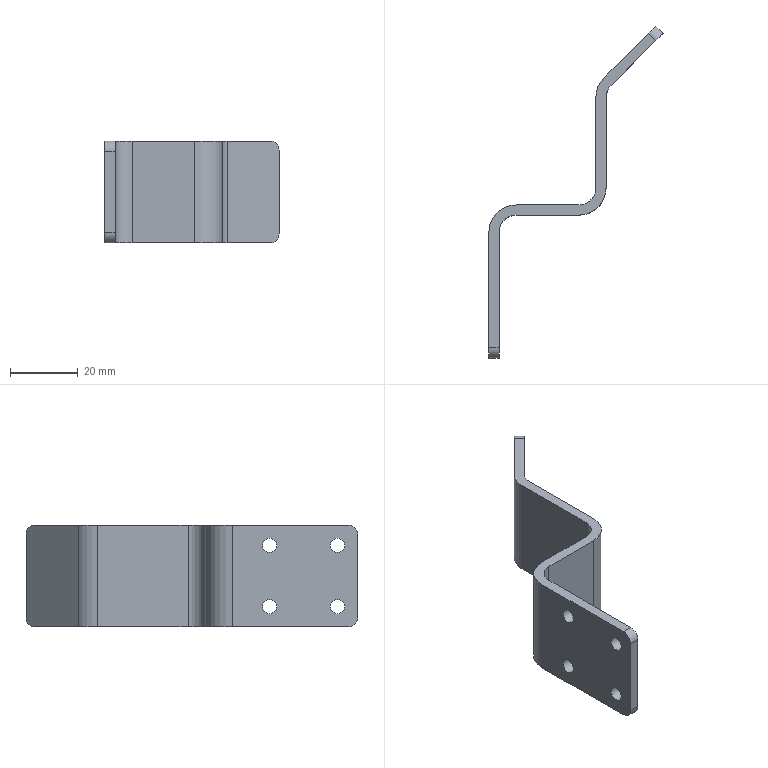Part | NX | features BREP 1 | 1 solid | 26 faces | box 51.299 x 97.678 x 30 mm | volume 11456 mm3 | cylinder 14 | plane 12 | commonest cylinder face diameters 4.2 x4 6 x4 10 x3 16 x3
STEP:
#1=CARTESIAN_POINT('',(-31.5,-50.,3.));
#2=VERTEX_POINT('',#1);
#3=CARTESIAN_POINT('',(-31.5,-47.,0.));
#4=VERTEX_POINT('',#3);
#5=CARTESIAN_POINT('',(-31.5,-47.,3.));
#6=DIRECTION('',(1.,0.,0.));
#7=DIRECTION('',(0.,1.,0.));
#8=AXIS2_PLACEMENT_3D('',#5,#6,#7);
#9=CIRCLE('',#8,3.);
#10=EDGE_CURVE('',#2,#4,#9,.T.);
#11=ORIENTED_EDGE('',*,*,#10,.F.);
#12=CARTESIAN_POINT('',(-31.5,-50.,27.));
#13=VERTEX_POINT('',#12);
#14=CARTESIAN_POINT('',(-31.5,-50.,0.));
#15=DIRECTION('',(0.,0.,-1.));
#16=VECTOR('',#15,1000.);
#17=LINE('',#14,#16);
#18=EDGE_CURVE('',#13,#2,#17,.T.);
#19=ORIENTED_EDGE('',*,*,#18,.F.);
#20=CARTESIAN_POINT('',(-31.5,-47.,30.));
#21=VERTEX_POINT('',#20);
#22=CARTESIAN_POINT('',(-31.5,-47.,27.));
#23=DIRECTION('',(1.,0.,0.));
#24=DIRECTION('',(0.,1.,0.));
#25=AXIS2_PLACEMENT_3D('',#22,#23,#24);
#26=CIRCLE('',#25,3.);
#27=EDGE_CURVE('',#21,#13,#26,.T.);
#28=ORIENTED_EDGE('',*,*,#27,.F.);
#29=CARTESIAN_POINT('',(-31.5,-13.,30.));
#30=VERTEX_POINT('',#29);
#31=CARTESIAN_POINT('',(-31.5,0.,30.));
#32=DIRECTION('',(0.,-1.,0.));
#33=VECTOR('',#32,1000.);
#34=LINE('',#31,#33);
#35=EDGE_CURVE('',#30,#21,#34,.T.);
#36=ORIENTED_EDGE('',*,*,#35,.F.);
#37=CARTESIAN_POINT('',(-31.5,-13.,0.));
#38=VERTEX_POINT('',#37);
#39=CARTESIAN_POINT('',(-31.5,-13.,0.));
#40=DIRECTION('',(0.,0.,1.));
#41=VECTOR('',#40,1000.);
#42=LINE('',#39,#41);
#43=EDGE_CURVE('',#38,#30,#42,.T.);
#44=ORIENTED_EDGE('',*,*,#43,.F.);
#45=CARTESIAN_POINT('',(-31.5,0.,0.));
#46=DIRECTION('',(0.,1.,0.));
#47=VECTOR('',#46,1000.);
#48=LINE('',#45,#47);
#49=EDGE_CURVE('',#4,#38,#48,.T.);
#50=ORIENTED_EDGE('',*,*,#49,.F.);
#51=EDGE_LOOP('',(#11,#19,#28,#36,#44,#50));
#52=FACE_BOUND('',#51,.T.);
#53=CARTESIAN_POINT('',(-31.5,-44.,26.1));
#54=VERTEX_POINT('',#53);
#55=CARTESIAN_POINT('',(-31.5,-44.,24.));
#56=DIRECTION('',(-1.,0.,0.));
#57=DIRECTION('',(0.,0.,1.));
#58=AXIS2_PLACEMENT_3D('',#55,#56,#57);
#59=CIRCLE('',#58,2.1);
#60=EDGE_CURVE('',#54,#54,#59,.T.);
#61=ORIENTED_EDGE('',*,*,#60,.F.);
#62=EDGE_LOOP('',(#61));
#63=FACE_BOUND('',#62,.T.);
#64=CARTESIAN_POINT('',(-31.5,-24.,26.1));
#65=VERTEX_POINT('',#64);
#66=CARTESIAN_POINT('',(-31.5,-24.,24.));
#67=DIRECTION('',(-1.,0.,0.));
#68=DIRECTION('',(0.,0.,1.));
#69=AXIS2_PLACEMENT_3D('',#66,#67,#68);
#70=CIRCLE('',#69,2.1);
#71=EDGE_CURVE('',#65,#65,#70,.T.);
#72=ORIENTED_EDGE('',*,*,#71,.F.);
#73=EDGE_LOOP('',(#72));
#74=FACE_BOUND('',#73,.T.);
#75=CARTESIAN_POINT('',(-31.5,-44.,8.1));
#76=VERTEX_POINT('',#75);
#77=CARTESIAN_POINT('',(-31.5,-44.,6.));
#78=DIRECTION('',(-1.,0.,0.));
#79=DIRECTION('',(0.,0.,1.));
#80=AXIS2_PLACEMENT_3D('',#77,#78,#79);
#81=CIRCLE('',#80,2.1);
#82=EDGE_CURVE('',#76,#76,#81,.T.);
#83=ORIENTED_EDGE('',*,*,#82,.F.);
#84=EDGE_LOOP('',(#83));
#85=FACE_BOUND('',#84,.T.);
#86=CARTESIAN_POINT('',(-31.5,-24.,8.1));
#87=VERTEX_POINT('',#86);
#88=CARTESIAN_POINT('',(-31.5,-24.,6.));
#89=DIRECTION('',(-1.,0.,0.));
#90=DIRECTION('',(0.,0.,1.));
#91=AXIS2_PLACEMENT_3D('',#88,#89,#90);
#92=CIRCLE('',#91,2.1);
#93=EDGE_CURVE('',#87,#87,#92,.T.);
#94=ORIENTED_EDGE('',*,*,#93,.F.);
#95=EDGE_LOOP('',(#94));
#96=FACE_BOUND('',#95,.T.);
#97=CARTESIAN_POINT('',(-31.5,0.,0.));
#98=DIRECTION('',(1.,0.,0.));
#99=DIRECTION('',(0.,0.,1.));
#100=AXIS2_PLACEMENT_3D('',#97,#98,#99);
#101=PLANE('',#100);
#102=ADVANCED_FACE('',(#52,#63,#74,#85,#96),#101,.F.);
#103=CARTESIAN_POINT('',(-28.5,-47.,0.));
#104=VERTEX_POINT('',#103);
#105=CARTESIAN_POINT('',(-31.5,-47.,0.));
#106=DIRECTION('',(1.,0.,0.));
#107=VECTOR('',#106,1000.);
#108=LINE('',#105,#107);
#109=EDGE_CURVE('',#4,#104,#108,.T.);
#110=ORIENTED_EDGE('',*,*,#109,.F.);
#111=ORIENTED_EDGE('',*,*,#49,.T.);
#112=CARTESIAN_POINT('',(-23.5,-5.,0.));
#113=VERTEX_POINT('',#112);
#114=CARTESIAN_POINT('',(-23.5,-13.,0.));
#115=DIRECTION('',(0.,0.,1.));
#116=DIRECTION('',(-1.,0.,0.));
#117=AXIS2_PLACEMENT_3D('',#114,#115,#116);
#118=CIRCLE('',#117,8.);
#119=EDGE_CURVE('',#113,#38,#118,.T.);
#120=ORIENTED_EDGE('',*,*,#119,.F.);
#121=CARTESIAN_POINT('',(-5.,-5.,0.));
#122=VERTEX_POINT('',#121);
#123=CARTESIAN_POINT('',(0.,-5.,0.));
#124=DIRECTION('',(-1.,0.,0.));
#125=VECTOR('',#124,1000.);
#126=LINE('',#123,#125);
#127=EDGE_CURVE('',#122,#113,#126,.T.);
#128=ORIENTED_EDGE('',*,*,#127,.F.);
#129=CARTESIAN_POINT('',(0.,0.,0.));
#130=VERTEX_POINT('',#129);
#131=CARTESIAN_POINT('',(-5.,0.,0.));
#132=DIRECTION('',(0.,0.,1.));
#133=DIRECTION('',(1.,0.,0.));
#134=AXIS2_PLACEMENT_3D('',#131,#132,#133);
#135=CIRCLE('',#134,5.);
#136=EDGE_CURVE('',#122,#130,#135,.T.);
#137=ORIENTED_EDGE('',*,*,#136,.T.);
#138=CARTESIAN_POINT('',(0.,26.686,0.));
#139=VERTEX_POINT('',#138);
#140=CARTESIAN_POINT('',(0.,0.,0.));
#141=DIRECTION('',(0.,-1.,0.));
#142=VECTOR('',#141,1000.);
#143=LINE('',#140,#142);
#144=EDGE_CURVE('',#139,#130,#143,.T.);
#145=ORIENTED_EDGE('',*,*,#144,.F.);
#146=CARTESIAN_POINT('',(2.343,32.343,0.));
#147=VERTEX_POINT('',#146);
#148=CARTESIAN_POINT('',(8.,26.686,0.));
#149=DIRECTION('',(0.,0.,1.));
#150=DIRECTION('',(-1.,0.,0.));
#151=AXIS2_PLACEMENT_3D('',#148,#149,#150);
#152=CIRCLE('',#151,8.);
#153=EDGE_CURVE('',#147,#139,#152,.T.);
#154=ORIENTED_EDGE('',*,*,#153,.F.);
#155=CARTESIAN_POINT('',(15.556,45.556,0.));
#156=VERTEX_POINT('',#155);
#157=CARTESIAN_POINT('',(0.,30.,0.));
#158=DIRECTION('',(-0.7071,-0.7071,0.));
#159=VECTOR('',#158,1000.);
#160=LINE('',#157,#159);
#161=EDGE_CURVE('',#156,#147,#160,.T.);
#162=ORIENTED_EDGE('',*,*,#161,.F.);
#163=CARTESIAN_POINT('',(17.678,43.435,0.));
#164=VERTEX_POINT('',#163);
#165=CARTESIAN_POINT('',(15.556,45.556,0.));
#166=DIRECTION('',(0.7071,-0.7071,0.));
#167=VECTOR('',#166,1000.);
#168=LINE('',#165,#167);
#169=EDGE_CURVE('',#156,#164,#168,.T.);
#170=ORIENTED_EDGE('',*,*,#169,.T.);
#171=CARTESIAN_POINT('',(4.464,30.222,0.));
#172=VERTEX_POINT('',#171);
#173=CARTESIAN_POINT('',(17.678,43.435,0.));
#174=DIRECTION('',(-0.7071,-0.7071,0.));
#175=VECTOR('',#174,1000.);
#176=LINE('',#173,#175);
#177=EDGE_CURVE('',#164,#172,#176,.T.);
#178=ORIENTED_EDGE('',*,*,#177,.T.);
#179=CARTESIAN_POINT('',(3.,26.686,0.));
#180=VERTEX_POINT('',#179);
#181=CARTESIAN_POINT('',(8.,26.686,0.));
#182=DIRECTION('',(0.,0.,1.));
#183=DIRECTION('',(-1.,0.,0.));
#184=AXIS2_PLACEMENT_3D('',#181,#182,#183);
#185=CIRCLE('',#184,5.);
#186=EDGE_CURVE('',#172,#180,#185,.T.);
#187=ORIENTED_EDGE('',*,*,#186,.T.);
#188=CARTESIAN_POINT('',(3.,0.,0.));
#189=VERTEX_POINT('',#188);
#190=CARTESIAN_POINT('',(3.,30.222,0.));
#191=DIRECTION('',(0.,-1.,0.));
#192=VECTOR('',#191,1000.);
#193=LINE('',#190,#192);
#194=EDGE_CURVE('',#180,#189,#193,.T.);
#195=ORIENTED_EDGE('',*,*,#194,.T.);
#196=CARTESIAN_POINT('',(-5.,-8.,0.));
#197=VERTEX_POINT('',#196);
#198=CARTESIAN_POINT('',(-5.,0.,0.));
#199=DIRECTION('',(0.,0.,-1.));
#200=DIRECTION('',(1.,0.,0.));
#201=AXIS2_PLACEMENT_3D('',#198,#199,#200);
#202=CIRCLE('',#201,8.);
#203=EDGE_CURVE('',#189,#197,#202,.T.);
#204=ORIENTED_EDGE('',*,*,#203,.T.);
#205=CARTESIAN_POINT('',(-23.5,-8.,0.));
#206=VERTEX_POINT('',#205);
#207=CARTESIAN_POINT('',(0.,-8.,0.));
#208=DIRECTION('',(1.,0.,0.));
#209=VECTOR('',#208,1000.);
#210=LINE('',#207,#209);
#211=EDGE_CURVE('',#206,#197,#210,.T.);
#212=ORIENTED_EDGE('',*,*,#211,.F.);
#213=CARTESIAN_POINT('',(-28.5,-13.,0.));
#214=VERTEX_POINT('',#213);
#215=CARTESIAN_POINT('',(-23.5,-13.,0.));
#216=DIRECTION('',(0.,0.,-1.));
#217=DIRECTION('',(-1.,0.,0.));
#218=AXIS2_PLACEMENT_3D('',#215,#216,#217);
#219=CIRCLE('',#218,5.);
#220=EDGE_CURVE('',#214,#206,#219,.T.);
#221=ORIENTED_EDGE('',*,*,#220,.F.);
#222=CARTESIAN_POINT('',(-28.5,-50.,0.));
#223=DIRECTION('',(0.,1.,0.));
#224=VECTOR('',#223,1000.);
#225=LINE('',#222,#224);
#226=EDGE_CURVE('',#104,#214,#225,.T.);
#227=ORIENTED_EDGE('',*,*,#226,.F.);
#228=EDGE_LOOP('',(#110,#111,#120,#128,#137,#145,#154,#162,#170,#178,#187,#195,#204,#212,#221,#227));
#229=FACE_BOUND('',#228,.T.);
#230=CARTESIAN_POINT('',(-31.5,-50.,0.));
#231=DIRECTION('',(0.,0.,1.));
#232=DIRECTION('',(-1.,0.,0.));
#233=AXIS2_PLACEMENT_3D('',#230,#231,#232);
#234=PLANE('',#233);
#235=ADVANCED_FACE('',(#229),#234,.F.);
#236=CARTESIAN_POINT('',(-28.5,-50.,3.));
#237=VERTEX_POINT('',#236);
#238=CARTESIAN_POINT('',(-28.5,-47.,3.));
#239=DIRECTION('',(-1.,0.,0.));
#240=DIRECTION('',(0.,1.,0.));
#241=AXIS2_PLACEMENT_3D('',#238,#239,#240);
#242=CIRCLE('',#241,3.);
#243=EDGE_CURVE('',#104,#237,#242,.T.);
#244=ORIENTED_EDGE('',*,*,#243,.T.);
#245=CARTESIAN_POINT('',(-31.5,-50.,3.));
#246=DIRECTION('',(-1.,0.,0.));
#247=VECTOR('',#246,1000.);
#248=LINE('',#245,#247);
#249=EDGE_CURVE('',#237,#2,#248,.T.);
#250=ORIENTED_EDGE('',*,*,#249,.T.);
#251=ORIENTED_EDGE('',*,*,#10,.T.);
#252=ORIENTED_EDGE('',*,*,#109,.T.);
#253=EDGE_LOOP('',(#244,#250,#251,#252));
#254=FACE_BOUND('',#253,.T.);
#255=CARTESIAN_POINT('',(-31.5,-47.,3.));
#256=DIRECTION('',(1.,0.,0.));
#257=DIRECTION('',(0.,-1.,0.));
#258=AXIS2_PLACEMENT_3D('',#255,#256,#257);
#259=CYLINDRICAL_SURFACE('',#258,3.);
#260=ADVANCED_FACE('',(#254),#259,.T.);
#261=ORIENTED_EDGE('',*,*,#249,.F.);
#262=CARTESIAN_POINT('',(-28.5,-50.,27.));
#263=VERTEX_POINT('',#262);
#264=CARTESIAN_POINT('',(-28.5,-50.,30.));
#265=DIRECTION('',(0.,0.,-1.));
#266=VECTOR('',#265,1000.);
#267=LINE('',#264,#266);
#268=EDGE_CURVE('',#263,#237,#267,.T.);
#269=ORIENTED_EDGE('',*,*,#268,.F.);
#270=CARTESIAN_POINT('',(-31.5,-50.,27.));
#271=DIRECTION('',(1.,0.,0.));
#272=VECTOR('',#271,1000.);
#273=LINE('',#270,#272);
#274=EDGE_CURVE('',#13,#263,#273,.T.);
#275=ORIENTED_EDGE('',*,*,#274,.F.);
#276=ORIENTED_EDGE('',*,*,#18,.T.);
#277=EDGE_LOOP('',(#261,#269,#275,#276));
#278=FACE_BOUND('',#277,.T.);
#279=CARTESIAN_POINT('',(-31.5,-50.,30.));
#280=DIRECTION('',(0.,1.,0.));
#281=DIRECTION('',(1.,0.,0.));
#282=AXIS2_PLACEMENT_3D('',#279,#280,#281);
#283=PLANE('',#282);
#284=ADVANCED_FACE('',(#278),#283,.F.);
#285=CARTESIAN_POINT('',(-28.5,-47.,30.));
#286=VERTEX_POINT('',#285);
#287=CARTESIAN_POINT('',(-28.5,-47.,27.));
#288=DIRECTION('',(-1.,0.,0.));
#289=DIRECTION('',(0.,1.,0.));
#290=AXIS2_PLACEMENT_3D('',#287,#288,#289);
#291=CIRCLE('',#290,3.);
#292=EDGE_CURVE('',#263,#286,#291,.T.);
#293=ORIENTED_EDGE('',*,*,#292,.T.);
#294=CARTESIAN_POINT('',(-31.5,-47.,30.));
#295=DIRECTION('',(-1.,0.,0.));
#296=VECTOR('',#295,1000.);
#297=LINE('',#294,#296);
#298=EDGE_CURVE('',#286,#21,#297,.T.);
#299=ORIENTED_EDGE('',*,*,#298,.T.);
#300=ORIENTED_EDGE('',*,*,#27,.T.);
#301=ORIENTED_EDGE('',*,*,#274,.T.);
#302=EDGE_LOOP('',(#293,#299,#300,#301));
#303=FACE_BOUND('',#302,.T.);
#304=CARTESIAN_POINT('',(-31.5,-47.,27.));
#305=DIRECTION('',(1.,0.,0.));
#306=DIRECTION('',(0.,-1.,0.));
#307=AXIS2_PLACEMENT_3D('',#304,#305,#306);
#308=CYLINDRICAL_SURFACE('',#307,3.);
#309=ADVANCED_FACE('',(#303),#308,.T.);
#310=ORIENTED_EDGE('',*,*,#298,.F.);
#311=CARTESIAN_POINT('',(-28.5,-13.,30.));
#312=VERTEX_POINT('',#311);
#313=CARTESIAN_POINT('',(-28.5,-8.,30.));
#314=DIRECTION('',(0.,-1.,0.));
#315=VECTOR('',#314,1000.);
#316=LINE('',#313,#315);
#317=EDGE_CURVE('',#312,#286,#316,.T.);
#318=ORIENTED_EDGE('',*,*,#317,.F.);
#319=CARTESIAN_POINT('',(-23.5,-8.,30.));
#320=VERTEX_POINT('',#319);
#321=CARTESIAN_POINT('',(-23.5,-13.,30.));
#322=DIRECTION('',(0.,0.,-1.));
#323=DIRECTION('',(-1.,0.,0.));
#324=AXIS2_PLACEMENT_3D('',#321,#322,#323);
#325=CIRCLE('',#324,5.);
#326=EDGE_CURVE('',#312,#320,#325,.T.);
#327=ORIENTED_EDGE('',*,*,#326,.T.);
#328=CARTESIAN_POINT('',(-5.,-8.,30.));
#329=VERTEX_POINT('',#328);
#330=CARTESIAN_POINT('',(-23.5,-8.,30.));
#331=DIRECTION('',(-1.,0.,0.));
#332=VECTOR('',#331,1000.);
#333=LINE('',#330,#332);
#334=EDGE_CURVE('',#329,#320,#333,.T.);
#335=ORIENTED_EDGE('',*,*,#334,.F.);
#336=CARTESIAN_POINT('',(3.,0.,30.));
#337=VERTEX_POINT('',#336);
#338=CARTESIAN_POINT('',(-5.,0.,30.));
#339=DIRECTION('',(0.,0.,-1.));
#340=DIRECTION('',(1.,0.,0.));
#341=AXIS2_PLACEMENT_3D('',#338,#339,#340);
#342=CIRCLE('',#341,8.);
#343=EDGE_CURVE('',#337,#329,#342,.T.);
#344=ORIENTED_EDGE('',*,*,#343,.F.);
#345=CARTESIAN_POINT('',(3.,26.686,30.));
#346=VERTEX_POINT('',#345);
#347=CARTESIAN_POINT('',(3.,26.686,30.));
#348=DIRECTION('',(0.,-1.,0.));
#349=VECTOR('',#348,1000.);
#350=LINE('',#347,#349);
#351=EDGE_CURVE('',#346,#337,#350,.T.);
#352=ORIENTED_EDGE('',*,*,#351,.F.);
#353=CARTESIAN_POINT('',(4.464,30.222,30.));
#354=VERTEX_POINT('',#353);
#355=CARTESIAN_POINT('',(8.,26.686,30.));
#356=DIRECTION('',(0.,0.,-1.));
#357=DIRECTION('',(-1.,0.,0.));
#358=AXIS2_PLACEMENT_3D('',#355,#356,#357);
#359=CIRCLE('',#358,5.);
#360=EDGE_CURVE('',#346,#354,#359,.T.);
#361=ORIENTED_EDGE('',*,*,#360,.T.);
#362=CARTESIAN_POINT('',(17.678,43.435,30.));
#363=VERTEX_POINT('',#362);
#364=CARTESIAN_POINT('',(4.464,30.222,30.));
#365=DIRECTION('',(0.7071,0.7071,0.));
#366=VECTOR('',#365,1000.);
#367=LINE('',#364,#366);
#368=EDGE_CURVE('',#354,#363,#367,.T.);
#369=ORIENTED_EDGE('',*,*,#368,.T.);
#370=CARTESIAN_POINT('',(15.556,45.556,30.));
#371=VERTEX_POINT('',#370);
#372=CARTESIAN_POINT('',(17.678,43.435,30.));
#373=DIRECTION('',(-0.7071,0.7071,0.));
#374=VECTOR('',#373,1000.);
#375=LINE('',#372,#374);
#376=EDGE_CURVE('',#363,#371,#375,.T.);
#377=ORIENTED_EDGE('',*,*,#376,.T.);
#378=CARTESIAN_POINT('',(2.343,32.343,30.));
#379=VERTEX_POINT('',#378);
#380=CARTESIAN_POINT('',(0.,30.,30.));
#381=DIRECTION('',(0.7071,0.7071,0.));
#382=VECTOR('',#381,1000.);
#383=LINE('',#380,#382);
#384=EDGE_CURVE('',#379,#371,#383,.T.);
#385=ORIENTED_EDGE('',*,*,#384,.F.);
#386=CARTESIAN_POINT('',(0.,26.686,30.));
#387=VERTEX_POINT('',#386);
#388=CARTESIAN_POINT('',(8.,26.686,30.));
#389=DIRECTION('',(0.,0.,-1.));
#390=DIRECTION('',(-1.,0.,0.));
#391=AXIS2_PLACEMENT_3D('',#388,#389,#390);
#392=CIRCLE('',#391,8.);
#393=EDGE_CURVE('',#387,#379,#392,.T.);
#394=ORIENTED_EDGE('',*,*,#393,.F.);
#395=CARTESIAN_POINT('',(0.,0.,30.));
#396=VERTEX_POINT('',#395);
#397=CARTESIAN_POINT('',(0.,0.,30.));
#398=DIRECTION('',(0.,1.,0.));
#399=VECTOR('',#398,1000.);
#400=LINE('',#397,#399);
#401=EDGE_CURVE('',#396,#387,#400,.T.);
#402=ORIENTED_EDGE('',*,*,#401,.F.);
#403=CARTESIAN_POINT('',(-5.,-5.,30.));
#404=VERTEX_POINT('',#403);
#405=CARTESIAN_POINT('',(-5.,0.,30.));
#406=DIRECTION('',(0.,0.,-1.));
#407=DIRECTION('',(1.,0.,0.));
#408=AXIS2_PLACEMENT_3D('',#405,#406,#407);
#409=CIRCLE('',#408,5.);
#410=EDGE_CURVE('',#396,#404,#409,.T.);
#411=ORIENTED_EDGE('',*,*,#410,.T.);
#412=CARTESIAN_POINT('',(-23.5,-5.,30.));
#413=VERTEX_POINT('',#412);
#414=CARTESIAN_POINT('',(0.,-5.,30.));
#415=DIRECTION('',(1.,0.,0.));
#416=VECTOR('',#415,1000.);
#417=LINE('',#414,#416);
#418=EDGE_CURVE('',#413,#404,#417,.T.);
#419=ORIENTED_EDGE('',*,*,#418,.F.);
#420=CARTESIAN_POINT('',(-23.5,-13.,30.));
#421=DIRECTION('',(0.,0.,-1.));
#422=DIRECTION('',(-1.,0.,0.));
#423=AXIS2_PLACEMENT_3D('',#420,#421,#422);
#424=CIRCLE('',#423,8.);
#425=EDGE_CURVE('',#30,#413,#424,.T.);
#426=ORIENTED_EDGE('',*,*,#425,.F.);
#427=ORIENTED_EDGE('',*,*,#35,.T.);
#428=EDGE_LOOP('',(#310,#318,#327,#335,#344,#352,#361,#369,#377,#385,#394,#402,#411,#419,#426,#427));
#429=FACE_BOUND('',#428,.T.);
#430=CARTESIAN_POINT('',(-31.5,-8.,30.));
#431=DIRECTION('',(0.,0.,-1.));
#432=DIRECTION('',(1.,0.,0.));
#433=AXIS2_PLACEMENT_3D('',#430,#431,#432);
#434=PLANE('',#433);
#435=ADVANCED_FACE('',(#429),#434,.F.);
#436=ORIENTED_EDGE('',*,*,#43,.T.);
#437=ORIENTED_EDGE('',*,*,#425,.T.);
#438=CARTESIAN_POINT('',(-23.5,-5.,0.));
#439=DIRECTION('',(0.,0.,-1.));
#440=VECTOR('',#439,1000.);
#441=LINE('',#438,#440);
#442=EDGE_CURVE('',#413,#113,#441,.T.);
#443=ORIENTED_EDGE('',*,*,#442,.T.);
#444=ORIENTED_EDGE('',*,*,#119,.T.);
#445=EDGE_LOOP('',(#436,#437,#443,#444));
#446=FACE_BOUND('',#445,.T.);
#447=CARTESIAN_POINT('',(-23.5,-13.,0.));
#448=DIRECTION('',(0.,0.,-1.));
#449=DIRECTION('',(1.,0.,0.));
#450=AXIS2_PLACEMENT_3D('',#447,#448,#449);
#451=CYLINDRICAL_SURFACE('',#450,8.);
#452=ADVANCED_FACE('',(#446),#451,.T.);
#453=CARTESIAN_POINT('',(-28.5,-44.,26.1));
#454=VERTEX_POINT('',#453);
#455=CARTESIAN_POINT('',(-28.5,-44.,24.));
#456=DIRECTION('',(-1.,0.,0.));
#457=DIRECTION('',(0.,0.,1.));
#458=AXIS2_PLACEMENT_3D('',#455,#456,#457);
#459=CIRCLE('',#458,2.1);
#460=EDGE_CURVE('',#454,#454,#459,.T.);
#461=ORIENTED_EDGE('',*,*,#460,.F.);
#462=EDGE_LOOP('',(#461));
#463=FACE_BOUND('',#462,.T.);
#464=ORIENTED_EDGE('',*,*,#60,.T.);
#465=EDGE_LOOP('',(#464));
#466=FACE_BOUND('',#465,.T.);
#467=CARTESIAN_POINT('',(-31.5,-44.,24.));
#468=DIRECTION('',(-1.,0.,0.));
#469=DIRECTION('',(0.,0.,-1.));
#470=AXIS2_PLACEMENT_3D('',#467,#468,#469);
#471=CYLINDRICAL_SURFACE('',#470,2.1);
#472=ADVANCED_FACE('',(#463,#466),#471,.F.);
#473=CARTESIAN_POINT('',(-28.5,-24.,26.1));
#474=VERTEX_POINT('',#473);
#475=CARTESIAN_POINT('',(-28.5,-24.,24.));
#476=DIRECTION('',(-1.,0.,0.));
#477=DIRECTION('',(0.,0.,1.));
#478=AXIS2_PLACEMENT_3D('',#475,#476,#477);
#479=CIRCLE('',#478,2.1);
#480=EDGE_CURVE('',#474,#474,#479,.T.);
#481=ORIENTED_EDGE('',*,*,#480,.F.);
#482=EDGE_LOOP('',(#481));
#483=FACE_BOUND('',#482,.T.);
#484=ORIENTED_EDGE('',*,*,#71,.T.);
#485=EDGE_LOOP('',(#484));
#486=FACE_BOUND('',#485,.T.);
#487=CARTESIAN_POINT('',(-31.5,-24.,24.));
#488=DIRECTION('',(-1.,0.,0.));
#489=DIRECTION('',(0.,0.,-1.));
#490=AXIS2_PLACEMENT_3D('',#487,#488,#489);
#491=CYLINDRICAL_SURFACE('',#490,2.1);
#492=ADVANCED_FACE('',(#483,#486),#491,.F.);
#493=CARTESIAN_POINT('',(-28.5,-44.,8.1));
#494=VERTEX_POINT('',#493);
#495=CARTESIAN_POINT('',(-28.5,-44.,6.));
#496=DIRECTION('',(-1.,0.,0.));
#497=DIRECTION('',(0.,0.,1.));
#498=AXIS2_PLACEMENT_3D('',#495,#496,#497);
#499=CIRCLE('',#498,2.1);
#500=EDGE_CURVE('',#494,#494,#499,.T.);
#501=ORIENTED_EDGE('',*,*,#500,.F.);
#502=EDGE_LOOP('',(#501));
#503=FACE_BOUND('',#502,.T.);
#504=ORIENTED_EDGE('',*,*,#82,.T.);
#505=EDGE_LOOP('',(#504));
#506=FACE_BOUND('',#505,.T.);
#507=CARTESIAN_POINT('',(-31.5,-44.,6.));
#508=DIRECTION('',(-1.,0.,0.));
#509=DIRECTION('',(0.,0.,-1.));
#510=AXIS2_PLACEMENT_3D('',#507,#508,#509);
#511=CYLINDRICAL_SURFACE('',#510,2.1);
#512=ADVANCED_FACE('',(#503,#506),#511,.F.);
#513=CARTESIAN_POINT('',(-28.5,-24.,8.1));
#514=VERTEX_POINT('',#513);
#515=CARTESIAN_POINT('',(-28.5,-24.,6.));
#516=DIRECTION('',(-1.,0.,0.));
#517=DIRECTION('',(0.,0.,1.));
#518=AXIS2_PLACEMENT_3D('',#515,#516,#517);
#519=CIRCLE('',#518,2.1);
#520=EDGE_CURVE('',#514,#514,#519,.T.);
#521=ORIENTED_EDGE('',*,*,#520,.F.);
#522=EDGE_LOOP('',(#521));
#523=FACE_BOUND('',#522,.T.);
#524=ORIENTED_EDGE('',*,*,#93,.T.);
#525=EDGE_LOOP('',(#524));
#526=FACE_BOUND('',#525,.T.);
#527=CARTESIAN_POINT('',(-31.5,-24.,6.));
#528=DIRECTION('',(-1.,0.,0.));
#529=DIRECTION('',(0.,0.,-1.));
#530=AXIS2_PLACEMENT_3D('',#527,#528,#529);
#531=CYLINDRICAL_SURFACE('',#530,2.1);
#532=ADVANCED_FACE('',(#523,#526),#531,.F.);
#533=ORIENTED_EDGE('',*,*,#317,.T.);
#534=ORIENTED_EDGE('',*,*,#292,.F.);
#535=ORIENTED_EDGE('',*,*,#268,.T.);
#536=ORIENTED_EDGE('',*,*,#243,.F.);
#537=ORIENTED_EDGE('',*,*,#226,.T.);
#538=CARTESIAN_POINT('',(-28.5,-13.,0.));
#539=DIRECTION('',(0.,0.,1.));
#540=VECTOR('',#539,1000.);
#541=LINE('',#538,#540);
#542=EDGE_CURVE('',#214,#312,#541,.T.);
#543=ORIENTED_EDGE('',*,*,#542,.T.);
#544=EDGE_LOOP('',(#533,#534,#535,#536,#537,#543));
#545=FACE_BOUND('',#544,.T.);
#546=ORIENTED_EDGE('',*,*,#460,.T.);
#547=EDGE_LOOP('',(#546));
#548=FACE_BOUND('',#547,.T.);
#549=ORIENTED_EDGE('',*,*,#480,.T.);
#550=EDGE_LOOP('',(#549));
#551=FACE_BOUND('',#550,.T.);
#552=ORIENTED_EDGE('',*,*,#500,.T.);
#553=EDGE_LOOP('',(#552));
#554=FACE_BOUND('',#553,.T.);
#555=ORIENTED_EDGE('',*,*,#520,.T.);
#556=EDGE_LOOP('',(#555));
#557=FACE_BOUND('',#556,.T.);
#558=CARTESIAN_POINT('',(-28.5,0.,0.));
#559=DIRECTION('',(1.,0.,0.));
#560=DIRECTION('',(0.,0.,1.));
#561=AXIS2_PLACEMENT_3D('',#558,#559,#560);
#562=PLANE('',#561);
#563=ADVANCED_FACE('',(#545,#548,#551,#554,#557),#562,.T.);
#564=ORIENTED_EDGE('',*,*,#127,.T.);
#565=ORIENTED_EDGE('',*,*,#442,.F.);
#566=ORIENTED_EDGE('',*,*,#418,.T.);
#567=CARTESIAN_POINT('',(-5.,-5.,0.));
#568=DIRECTION('',(0.,0.,-1.));
#569=VECTOR('',#568,1000.);
#570=LINE('',#567,#569);
#571=EDGE_CURVE('',#404,#122,#570,.T.);
#572=ORIENTED_EDGE('',*,*,#571,.T.);
#573=EDGE_LOOP('',(#564,#565,#566,#572));
#574=FACE_BOUND('',#573,.T.);
#575=CARTESIAN_POINT('',(0.,-5.,0.));
#576=DIRECTION('',(0.,1.,0.));
#577=DIRECTION('',(1.,0.,0.));
#578=AXIS2_PLACEMENT_3D('',#575,#576,#577);
#579=PLANE('',#578);
#580=ADVANCED_FACE('',(#574),#579,.T.);
#581=ORIENTED_EDGE('',*,*,#326,.F.);
#582=ORIENTED_EDGE('',*,*,#542,.F.);
#583=ORIENTED_EDGE('',*,*,#220,.T.);
#584=CARTESIAN_POINT('',(-23.5,-8.,0.));
#585=DIRECTION('',(0.,0.,-1.));
#586=VECTOR('',#585,1000.);
#587=LINE('',#584,#586);
#588=EDGE_CURVE('',#320,#206,#587,.T.);
#589=ORIENTED_EDGE('',*,*,#588,.F.);
#590=EDGE_LOOP('',(#581,#582,#583,#589));
#591=FACE_BOUND('',#590,.T.);
#592=CARTESIAN_POINT('',(-23.5,-13.,0.));
#593=DIRECTION('',(0.,0.,-1.));
#594=DIRECTION('',(1.,0.,0.));
#595=AXIS2_PLACEMENT_3D('',#592,#593,#594);
#596=CYLINDRICAL_SURFACE('',#595,5.);
#597=ADVANCED_FACE('',(#591),#596,.F.);
#598=ORIENTED_EDGE('',*,*,#136,.F.);
#599=ORIENTED_EDGE('',*,*,#571,.F.);
#600=ORIENTED_EDGE('',*,*,#410,.F.);
#601=CARTESIAN_POINT('',(0.,0.,30.));
#602=DIRECTION('',(0.,0.,1.));
#603=VECTOR('',#602,1000.);
#604=LINE('',#601,#603);
#605=EDGE_CURVE('',#130,#396,#604,.T.);
#606=ORIENTED_EDGE('',*,*,#605,.F.);
#607=EDGE_LOOP('',(#598,#599,#600,#606));
#608=FACE_BOUND('',#607,.T.);
#609=CARTESIAN_POINT('',(-5.,0.,30.));
#610=DIRECTION('',(0.,0.,1.));
#611=DIRECTION('',(-1.,0.,0.));
#612=AXIS2_PLACEMENT_3D('',#609,#610,#611);
#613=CYLINDRICAL_SURFACE('',#612,5.);
#614=ADVANCED_FACE('',(#608),#613,.F.);
#615=ORIENTED_EDGE('',*,*,#334,.T.);
#616=ORIENTED_EDGE('',*,*,#588,.T.);
#617=ORIENTED_EDGE('',*,*,#211,.T.);
#618=CARTESIAN_POINT('',(-5.,-8.,0.));
#619=DIRECTION('',(0.,0.,-1.));
#620=VECTOR('',#619,1000.);
#621=LINE('',#618,#620);
#622=EDGE_CURVE('',#329,#197,#621,.T.);
#623=ORIENTED_EDGE('',*,*,#622,.F.);
#624=EDGE_LOOP('',(#615,#616,#617,#623));
#625=FACE_BOUND('',#624,.T.);
#626=CARTESIAN_POINT('',(0.,-8.,0.));
#627=DIRECTION('',(0.,1.,0.));
#628=DIRECTION('',(1.,0.,0.));
#629=AXIS2_PLACEMENT_3D('',#626,#627,#628);
#630=PLANE('',#629);
#631=ADVANCED_FACE('',(#625),#630,.F.);
#632=ORIENTED_EDGE('',*,*,#401,.T.);
#633=CARTESIAN_POINT('',(0.,26.686,30.));
#634=DIRECTION('',(0.,0.,-1.));
#635=VECTOR('',#634,1000.);
#636=LINE('',#633,#635);
#637=EDGE_CURVE('',#387,#139,#636,.T.);
#638=ORIENTED_EDGE('',*,*,#637,.T.);
#639=ORIENTED_EDGE('',*,*,#144,.T.);
#640=ORIENTED_EDGE('',*,*,#605,.T.);
#641=EDGE_LOOP('',(#632,#638,#639,#640));
#642=FACE_BOUND('',#641,.T.);
#643=CARTESIAN_POINT('',(0.,0.,30.));
#644=DIRECTION('',(-1.,0.,0.));
#645=DIRECTION('',(0.,0.,-1.));
#646=AXIS2_PLACEMENT_3D('',#643,#644,#645);
#647=PLANE('',#646);
#648=ADVANCED_FACE('',(#642),#647,.T.);
#649=ORIENTED_EDGE('',*,*,#622,.T.);
#650=ORIENTED_EDGE('',*,*,#203,.F.);
#651=CARTESIAN_POINT('',(3.,0.,30.));
#652=DIRECTION('',(0.,0.,1.));
#653=VECTOR('',#652,1000.);
#654=LINE('',#651,#653);
#655=EDGE_CURVE('',#189,#337,#654,.T.);
#656=ORIENTED_EDGE('',*,*,#655,.T.);
#657=ORIENTED_EDGE('',*,*,#343,.T.);
#658=EDGE_LOOP('',(#649,#650,#656,#657));
#659=FACE_BOUND('',#658,.T.);
#660=CARTESIAN_POINT('',(-5.,0.,30.));
#661=DIRECTION('',(0.,0.,1.));
#662=DIRECTION('',(-1.,0.,0.));
#663=AXIS2_PLACEMENT_3D('',#660,#661,#662);
#664=CYLINDRICAL_SURFACE('',#663,8.);
#665=ADVANCED_FACE('',(#659),#664,.T.);
#666=ORIENTED_EDGE('',*,*,#393,.T.);
#667=CARTESIAN_POINT('',(2.343,32.343,30.));
#668=DIRECTION('',(0.,0.,-1.));
#669=VECTOR('',#668,1000.);
#670=LINE('',#667,#669);
#671=EDGE_CURVE('',#379,#147,#670,.T.);
#672=ORIENTED_EDGE('',*,*,#671,.T.);
#673=ORIENTED_EDGE('',*,*,#153,.T.);
#674=ORIENTED_EDGE('',*,*,#637,.F.);
#675=EDGE_LOOP('',(#666,#672,#673,#674));
#676=FACE_BOUND('',#675,.T.);
#677=CARTESIAN_POINT('',(8.,26.686,30.));
#678=DIRECTION('',(0.,0.,-1.));
#679=DIRECTION('',(1.,0.,0.));
#680=AXIS2_PLACEMENT_3D('',#677,#678,#679);
#681=CYLINDRICAL_SURFACE('',#680,8.);
#682=ADVANCED_FACE('',(#676),#681,.T.);
#683=CARTESIAN_POINT('',(3.,26.686,30.));
#684=DIRECTION('',(0.,0.,-1.));
#685=VECTOR('',#684,1000.);
#686=LINE('',#683,#685);
#687=EDGE_CURVE('',#346,#180,#686,.T.);
#688=ORIENTED_EDGE('',*,*,#687,.F.);
#689=ORIENTED_EDGE('',*,*,#351,.T.);
#690=ORIENTED_EDGE('',*,*,#655,.F.);
#691=ORIENTED_EDGE('',*,*,#194,.F.);
#692=EDGE_LOOP('',(#688,#689,#690,#691));
#693=FACE_BOUND('',#692,.T.);
#694=CARTESIAN_POINT('',(3.,0.,30.));
#695=DIRECTION('',(-1.,0.,0.));
#696=DIRECTION('',(0.,0.,-1.));
#697=AXIS2_PLACEMENT_3D('',#694,#695,#696);
#698=PLANE('',#697);
#699=ADVANCED_FACE('',(#693),#698,.F.);
#700=ORIENTED_EDGE('',*,*,#384,.T.);
#701=CARTESIAN_POINT('',(17.678,47.678,27.));
#702=VERTEX_POINT('',#701);
#703=CARTESIAN_POINT('',(15.556,45.556,27.));
#704=DIRECTION('',(-0.7071,0.7071,0.));
#705=DIRECTION('',(0.7071,0.7071,0.));
#706=AXIS2_PLACEMENT_3D('',#703,#704,#705);
#707=CIRCLE('',#706,3.);
#708=EDGE_CURVE('',#371,#702,#707,.T.);
#709=ORIENTED_EDGE('',*,*,#708,.T.);
#710=CARTESIAN_POINT('',(17.678,47.678,3.));
#711=VERTEX_POINT('',#710);
#712=CARTESIAN_POINT('',(17.678,47.678,30.));
#713=DIRECTION('',(0.,0.,-1.));
#714=VECTOR('',#713,1000.);
#715=LINE('',#712,#714);
#716=EDGE_CURVE('',#702,#711,#715,.T.);
#717=ORIENTED_EDGE('',*,*,#716,.T.);
#718=CARTESIAN_POINT('',(15.556,45.556,3.));
#719=DIRECTION('',(-0.7071,0.7071,0.));
#720=DIRECTION('',(0.7071,0.7071,0.));
#721=AXIS2_PLACEMENT_3D('',#718,#719,#720);
#722=CIRCLE('',#721,3.);
#723=EDGE_CURVE('',#711,#156,#722,.T.);
#724=ORIENTED_EDGE('',*,*,#723,.T.);
#725=ORIENTED_EDGE('',*,*,#161,.T.);
#726=ORIENTED_EDGE('',*,*,#671,.F.);
#727=EDGE_LOOP('',(#700,#709,#717,#724,#725,#726));
#728=FACE_BOUND('',#727,.T.);
#729=CARTESIAN_POINT('',(0.,30.,30.));
#730=DIRECTION('',(-0.7071,0.7071,0.));
#731=DIRECTION('',(0.7071,0.7071,0.));
#732=AXIS2_PLACEMENT_3D('',#729,#730,#731);
#733=PLANE('',#732);
#734=ADVANCED_FACE('',(#728),#733,.T.);
#735=CARTESIAN_POINT('',(4.464,30.222,30.));
#736=DIRECTION('',(0.,0.,-1.));
#737=VECTOR('',#736,1000.);
#738=LINE('',#735,#737);
#739=EDGE_CURVE('',#354,#172,#738,.T.);
#740=ORIENTED_EDGE('',*,*,#739,.F.);
#741=ORIENTED_EDGE('',*,*,#360,.F.);
#742=ORIENTED_EDGE('',*,*,#687,.T.);
#743=ORIENTED_EDGE('',*,*,#186,.F.);
#744=EDGE_LOOP('',(#740,#741,#742,#743));
#745=FACE_BOUND('',#744,.T.);
#746=CARTESIAN_POINT('',(8.,26.686,30.));
#747=DIRECTION('',(0.,0.,-1.));
#748=DIRECTION('',(1.,0.,0.));
#749=AXIS2_PLACEMENT_3D('',#746,#747,#748);
#750=CYLINDRICAL_SURFACE('',#749,5.);
#751=ADVANCED_FACE('',(#745),#750,.F.);
#752=CARTESIAN_POINT('',(19.799,45.556,27.));
#753=VERTEX_POINT('',#752);
#754=CARTESIAN_POINT('',(17.678,43.435,27.));
#755=DIRECTION('',(-0.7071,0.7071,0.));
#756=DIRECTION('',(0.7071,0.7071,0.));
#757=AXIS2_PLACEMENT_3D('',#754,#755,#756);
#758=CIRCLE('',#757,3.);
#759=EDGE_CURVE('',#363,#753,#758,.T.);
#760=ORIENTED_EDGE('',*,*,#759,.T.);
#761=CARTESIAN_POINT('',(17.678,47.678,27.));
#762=DIRECTION('',(-0.7071,0.7071,0.));
#763=VECTOR('',#762,1000.);
#764=LINE('',#761,#763);
#765=EDGE_CURVE('',#753,#702,#764,.T.);
#766=ORIENTED_EDGE('',*,*,#765,.T.);
#767=ORIENTED_EDGE('',*,*,#708,.F.);
#768=ORIENTED_EDGE('',*,*,#376,.F.);
#769=EDGE_LOOP('',(#760,#766,#767,#768));
#770=FACE_BOUND('',#769,.T.);
#771=CARTESIAN_POINT('',(15.556,45.556,27.));
#772=DIRECTION('',(0.7071,-0.7071,0.));
#773=DIRECTION('',(-0.7071,-0.7071,0.));
#774=AXIS2_PLACEMENT_3D('',#771,#772,#773);
#775=CYLINDRICAL_SURFACE('',#774,3.);
#776=ADVANCED_FACE('',(#770),#775,.T.);
#777=CARTESIAN_POINT('',(19.799,45.556,3.));
#778=VERTEX_POINT('',#777);
#779=CARTESIAN_POINT('',(17.678,43.435,3.));
#780=DIRECTION('',(-0.7071,0.7071,0.));
#781=DIRECTION('',(0.7071,0.7071,0.));
#782=AXIS2_PLACEMENT_3D('',#779,#780,#781);
#783=CIRCLE('',#782,3.);
#784=EDGE_CURVE('',#778,#164,#783,.T.);
#785=ORIENTED_EDGE('',*,*,#784,.T.);
#786=ORIENTED_EDGE('',*,*,#169,.F.);
#787=ORIENTED_EDGE('',*,*,#723,.F.);
#788=CARTESIAN_POINT('',(23.335,42.021,3.));
#789=DIRECTION('',(0.7071,-0.7071,0.));
#790=VECTOR('',#789,1000.);
#791=LINE('',#788,#790);
#792=EDGE_CURVE('',#711,#778,#791,.T.);
#793=ORIENTED_EDGE('',*,*,#792,.T.);
#794=EDGE_LOOP('',(#785,#786,#787,#793));
#795=FACE_BOUND('',#794,.T.);
#796=CARTESIAN_POINT('',(21.213,39.899,3.));
#797=DIRECTION('',(0.7071,-0.7071,0.));
#798=DIRECTION('',(-0.7071,-0.7071,0.));
#799=AXIS2_PLACEMENT_3D('',#796,#797,#798);
#800=CYLINDRICAL_SURFACE('',#799,3.);
#801=ADVANCED_FACE('',(#795),#800,.T.);
#802=ORIENTED_EDGE('',*,*,#716,.F.);
#803=ORIENTED_EDGE('',*,*,#765,.F.);
#804=CARTESIAN_POINT('',(19.799,45.556,30.));
#805=DIRECTION('',(0.,0.,-1.));
#806=VECTOR('',#805,1000.);
#807=LINE('',#804,#806);
#808=EDGE_CURVE('',#753,#778,#807,.T.);
#809=ORIENTED_EDGE('',*,*,#808,.T.);
#810=ORIENTED_EDGE('',*,*,#792,.F.);
#811=EDGE_LOOP('',(#802,#803,#809,#810));
#812=FACE_BOUND('',#811,.T.);
#813=CARTESIAN_POINT('',(17.678,47.678,30.));
#814=DIRECTION('',(0.7071,0.7071,0.));
#815=DIRECTION('',(0.7071,-0.7071,0.));
#816=AXIS2_PLACEMENT_3D('',#813,#814,#815);
#817=PLANE('',#816);
#818=ADVANCED_FACE('',(#812),#817,.T.);
#819=ORIENTED_EDGE('',*,*,#784,.F.);
#820=ORIENTED_EDGE('',*,*,#808,.F.);
#821=ORIENTED_EDGE('',*,*,#759,.F.);
#822=ORIENTED_EDGE('',*,*,#368,.F.);
#823=ORIENTED_EDGE('',*,*,#739,.T.);
#824=ORIENTED_EDGE('',*,*,#177,.F.);
#825=EDGE_LOOP('',(#819,#820,#821,#822,#823,#824));
#826=FACE_BOUND('',#825,.T.);
#827=CARTESIAN_POINT('',(2.121,27.879,30.));
#828=DIRECTION('',(-0.7071,0.7071,0.));
#829=DIRECTION('',(0.7071,0.7071,0.));
#830=AXIS2_PLACEMENT_3D('',#827,#828,#829);
#831=PLANE('',#830);
#832=ADVANCED_FACE('',(#826),#831,.F.);
#833=CLOSED_SHELL('',(#102,#235,#260,#284,#309,#435,#452,#472,#492,#512,#532,#563,#580,#597,#614,#631,#648,#665,#682,#699,#734,#751,#776,#801,#818,#832));
#834=MANIFOLD_SOLID_BREP('',#833);
#835=(LENGTH_UNIT()NAMED_UNIT(*)SI_UNIT(.MILLI.,.METRE.));
#836=UNCERTAINTY_MEASURE_WITH_UNIT(LENGTH_MEASURE(0.00001),#835,'','');
#837=(NAMED_UNIT(*)PLANE_ANGLE_UNIT()SI_UNIT($,.RADIAN.));
#838=(NAMED_UNIT(*)SI_UNIT($,.STERADIAN.)SOLID_ANGLE_UNIT());
#839=(GEOMETRIC_REPRESENTATION_CONTEXT(3)GLOBAL_UNCERTAINTY_ASSIGNED_CONTEXT((#836))GLOBAL_UNIT_ASSIGNED_CONTEXT((#835,#837,#838))REPRESENTATION_CONTEXT('',''));
#840=ADVANCED_BREP_SHAPE_REPRESENTATION('',(#834),#839);